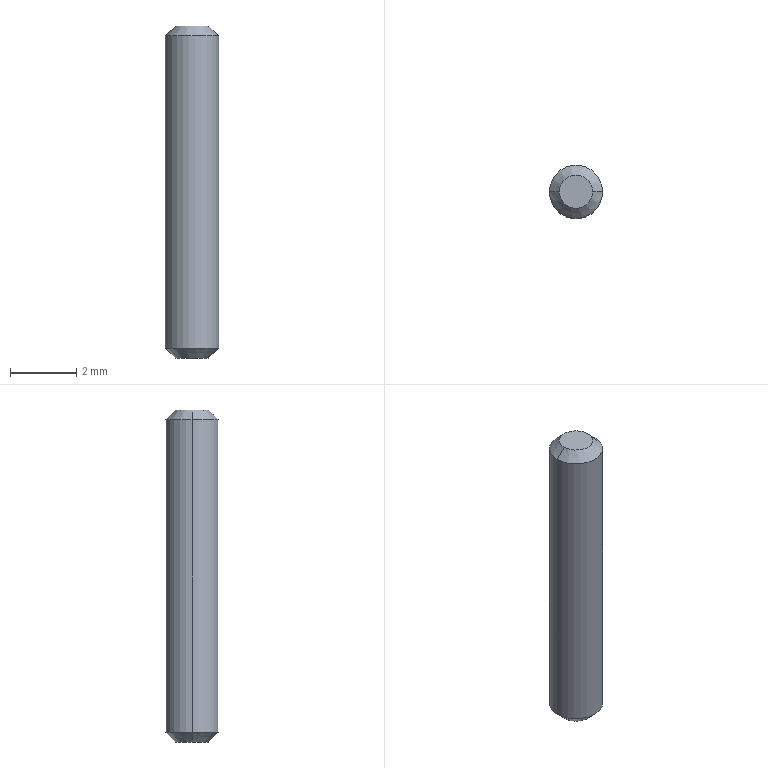Part | STEP file | 1 solid | 8 faces | box 1.6 x 1.6 x 10 mm | volume 19.71 mm3 | cone 4 | cylinder 2 | plane 2 | commonest cylinder face diameters 1.6 x2
STEP:
#1=CARTESIAN_POINT('',(-0.8,0.,9.7));
#2=VERTEX_POINT('',#1);
#3=CARTESIAN_POINT('',(0.8,0.,9.7));
#4=VERTEX_POINT('',#3);
#5=CARTESIAN_POINT('',(0.,0.,9.7));
#6=DIRECTION('',(0.,0.,-1.));
#7=DIRECTION('',(-1.,0.,0.));
#8=AXIS2_PLACEMENT_3D('',#5,#6,#7);
#9=CIRCLE('',#8,0.8);
#10=EDGE_CURVE('',#2,#4,#9,.T.);
#11=ORIENTED_EDGE('',*,*,#10,.T.);
#12=CARTESIAN_POINT('',(0.8,0.,0.3));
#13=VERTEX_POINT('',#12);
#14=CARTESIAN_POINT('',(0.8,0.,10.));
#15=DIRECTION('',(0.,0.,-1.));
#16=VECTOR('',#15,1000.);
#17=LINE('',#14,#16);
#18=EDGE_CURVE('',#4,#13,#17,.T.);
#19=ORIENTED_EDGE('',*,*,#18,.T.);
#20=CARTESIAN_POINT('',(-0.8,0.,0.3));
#21=VERTEX_POINT('',#20);
#22=CARTESIAN_POINT('',(0.,0.,0.3));
#23=DIRECTION('',(0.,0.,1.));
#24=DIRECTION('',(-1.,0.,0.));
#25=AXIS2_PLACEMENT_3D('',#22,#23,#24);
#26=CIRCLE('',#25,0.8);
#27=EDGE_CURVE('',#13,#21,#26,.T.);
#28=ORIENTED_EDGE('',*,*,#27,.T.);
#29=CARTESIAN_POINT('',(-0.8,0.,10.));
#30=DIRECTION('',(0.,0.,-1.));
#31=VECTOR('',#30,1000.);
#32=LINE('',#29,#31);
#33=EDGE_CURVE('',#2,#21,#32,.T.);
#34=ORIENTED_EDGE('',*,*,#33,.F.);
#35=EDGE_LOOP('',(#11,#19,#28,#34));
#36=FACE_OUTER_BOUND('',#35,.T.);
#37=CARTESIAN_POINT('',(0.,0.,10.));
#38=DIRECTION('',(0.,0.,-1.));
#39=DIRECTION('',(-1.,0.,0.));
#40=AXIS2_PLACEMENT_3D('',#37,#38,#39);
#41=CYLINDRICAL_SURFACE('',#40,0.8);
#42=ADVANCED_FACE('',(#36),#41,.T.);
#43=CARTESIAN_POINT('',(0.5,0.,0.));
#44=VERTEX_POINT('',#43);
#45=CARTESIAN_POINT('',(-0.5,0.,0.));
#46=VERTEX_POINT('',#45);
#47=CARTESIAN_POINT('',(0.,0.,0.));
#48=DIRECTION('',(0.,0.,1.));
#49=DIRECTION('',(1.,0.,0.));
#50=AXIS2_PLACEMENT_3D('',#47,#48,#49);
#51=CIRCLE('',#50,0.5);
#52=EDGE_CURVE('',#44,#46,#51,.T.);
#53=ORIENTED_EDGE('',*,*,#52,.T.);
#54=CARTESIAN_POINT('',(-0.8,0.,0.3));
#55=DIRECTION('',(-0.7071,0.,0.7071));
#56=VECTOR('',#55,1000.);
#57=LINE('',#54,#56);
#58=EDGE_CURVE('',#46,#21,#57,.T.);
#59=ORIENTED_EDGE('',*,*,#58,.T.);
#60=ORIENTED_EDGE('',*,*,#27,.F.);
#61=CARTESIAN_POINT('',(0.8,0.,0.3));
#62=DIRECTION('',(0.7071,0.,0.7071));
#63=VECTOR('',#62,1000.);
#64=LINE('',#61,#63);
#65=EDGE_CURVE('',#44,#13,#64,.T.);
#66=ORIENTED_EDGE('',*,*,#65,.F.);
#67=EDGE_LOOP('',(#53,#59,#60,#66));
#68=FACE_OUTER_BOUND('',#67,.T.);
#69=CARTESIAN_POINT('',(0.,0.,0.3));
#70=DIRECTION('',(0.,0.,1.));
#71=DIRECTION('',(1.,0.,0.));
#72=AXIS2_PLACEMENT_3D('',#69,#70,#71);
#73=CONICAL_SURFACE('',#72,0.8,0.7854);
#74=ADVANCED_FACE('',(#68),#73,.T.);
#75=CARTESIAN_POINT('',(-0.5,0.,10.));
#76=VERTEX_POINT('',#75);
#77=CARTESIAN_POINT('',(0.5,0.,10.));
#78=VERTEX_POINT('',#77);
#79=CARTESIAN_POINT('',(0.,0.,10.));
#80=DIRECTION('',(0.,0.,-1.));
#81=DIRECTION('',(-1.,0.,0.));
#82=AXIS2_PLACEMENT_3D('',#79,#80,#81);
#83=CIRCLE('',#82,0.5);
#84=EDGE_CURVE('',#76,#78,#83,.T.);
#85=ORIENTED_EDGE('',*,*,#84,.T.);
#86=CARTESIAN_POINT('',(0.8,0.,9.7));
#87=DIRECTION('',(0.7071,0.,-0.7071));
#88=VECTOR('',#87,1000.);
#89=LINE('',#86,#88);
#90=EDGE_CURVE('',#78,#4,#89,.T.);
#91=ORIENTED_EDGE('',*,*,#90,.T.);
#92=ORIENTED_EDGE('',*,*,#10,.F.);
#93=CARTESIAN_POINT('',(-0.8,0.,9.7));
#94=DIRECTION('',(-0.7071,0.,-0.7071));
#95=VECTOR('',#94,1000.);
#96=LINE('',#93,#95);
#97=EDGE_CURVE('',#76,#2,#96,.T.);
#98=ORIENTED_EDGE('',*,*,#97,.F.);
#99=EDGE_LOOP('',(#85,#91,#92,#98));
#100=FACE_OUTER_BOUND('',#99,.T.);
#101=CARTESIAN_POINT('',(0.,0.,9.7));
#102=DIRECTION('',(0.,0.,-1.));
#103=DIRECTION('',(-1.,0.,0.));
#104=AXIS2_PLACEMENT_3D('',#101,#102,#103);
#105=CONICAL_SURFACE('',#104,0.8,0.7854);
#106=ADVANCED_FACE('',(#100),#105,.T.);
#107=ORIENTED_EDGE('',*,*,#18,.F.);
#108=CARTESIAN_POINT('',(0.,0.,9.7));
#109=DIRECTION('',(0.,0.,-1.));
#110=DIRECTION('',(-1.,0.,0.));
#111=AXIS2_PLACEMENT_3D('',#108,#109,#110);
#112=CIRCLE('',#111,0.8);
#113=EDGE_CURVE('',#4,#2,#112,.T.);
#114=ORIENTED_EDGE('',*,*,#113,.T.);
#115=ORIENTED_EDGE('',*,*,#33,.T.);
#116=CARTESIAN_POINT('',(0.,0.,0.3));
#117=DIRECTION('',(0.,0.,1.));
#118=DIRECTION('',(-1.,0.,0.));
#119=AXIS2_PLACEMENT_3D('',#116,#117,#118);
#120=CIRCLE('',#119,0.8);
#121=EDGE_CURVE('',#21,#13,#120,.T.);
#122=ORIENTED_EDGE('',*,*,#121,.T.);
#123=EDGE_LOOP('',(#107,#114,#115,#122));
#124=FACE_OUTER_BOUND('',#123,.T.);
#125=CARTESIAN_POINT('',(0.,0.,10.));
#126=DIRECTION('',(0.,0.,-1.));
#127=DIRECTION('',(-1.,0.,0.));
#128=AXIS2_PLACEMENT_3D('',#125,#126,#127);
#129=CYLINDRICAL_SURFACE('',#128,0.8);
#130=ADVANCED_FACE('',(#124),#129,.T.);
#131=ORIENTED_EDGE('',*,*,#58,.F.);
#132=CARTESIAN_POINT('',(0.,0.,0.));
#133=DIRECTION('',(0.,0.,1.));
#134=DIRECTION('',(1.,0.,0.));
#135=AXIS2_PLACEMENT_3D('',#132,#133,#134);
#136=CIRCLE('',#135,0.5);
#137=EDGE_CURVE('',#46,#44,#136,.T.);
#138=ORIENTED_EDGE('',*,*,#137,.T.);
#139=ORIENTED_EDGE('',*,*,#65,.T.);
#140=ORIENTED_EDGE('',*,*,#121,.F.);
#141=EDGE_LOOP('',(#131,#138,#139,#140));
#142=FACE_OUTER_BOUND('',#141,.T.);
#143=CARTESIAN_POINT('',(0.,0.,0.3));
#144=DIRECTION('',(0.,0.,1.));
#145=DIRECTION('',(1.,0.,0.));
#146=AXIS2_PLACEMENT_3D('',#143,#144,#145);
#147=CONICAL_SURFACE('',#146,0.8,0.7854);
#148=ADVANCED_FACE('',(#142),#147,.T.);
#149=ORIENTED_EDGE('',*,*,#90,.F.);
#150=CARTESIAN_POINT('',(0.,0.,10.));
#151=DIRECTION('',(0.,0.,-1.));
#152=DIRECTION('',(-1.,0.,0.));
#153=AXIS2_PLACEMENT_3D('',#150,#151,#152);
#154=CIRCLE('',#153,0.5);
#155=EDGE_CURVE('',#78,#76,#154,.T.);
#156=ORIENTED_EDGE('',*,*,#155,.T.);
#157=ORIENTED_EDGE('',*,*,#97,.T.);
#158=ORIENTED_EDGE('',*,*,#113,.F.);
#159=EDGE_LOOP('',(#149,#156,#157,#158));
#160=FACE_OUTER_BOUND('',#159,.T.);
#161=CARTESIAN_POINT('',(0.,0.,9.7));
#162=DIRECTION('',(0.,0.,-1.));
#163=DIRECTION('',(-1.,0.,0.));
#164=AXIS2_PLACEMENT_3D('',#161,#162,#163);
#165=CONICAL_SURFACE('',#164,0.8,0.7854);
#166=ADVANCED_FACE('',(#160),#165,.T.);
#167=ORIENTED_EDGE('',*,*,#52,.F.);
#168=ORIENTED_EDGE('',*,*,#137,.F.);
#169=EDGE_LOOP('',(#167,#168));
#170=FACE_OUTER_BOUND('',#169,.T.);
#171=CARTESIAN_POINT('',(0.,0.,0.));
#172=DIRECTION('',(0.,0.,1.));
#173=DIRECTION('',(1.,0.,0.));
#174=AXIS2_PLACEMENT_3D('',#171,#172,#173);
#175=PLANE('',#174);
#176=ADVANCED_FACE('',(#170),#175,.F.);
#177=ORIENTED_EDGE('',*,*,#84,.F.);
#178=ORIENTED_EDGE('',*,*,#155,.F.);
#179=EDGE_LOOP('',(#177,#178));
#180=FACE_OUTER_BOUND('',#179,.T.);
#181=CARTESIAN_POINT('',(0.,0.,10.));
#182=DIRECTION('',(0.,0.,1.));
#183=DIRECTION('',(1.,0.,0.));
#184=AXIS2_PLACEMENT_3D('',#181,#182,#183);
#185=PLANE('',#184);
#186=ADVANCED_FACE('',(#180),#185,.T.);
#187=CLOSED_SHELL('',(#42,#74,#106,#130,#148,#166,#176,#186));
#188=MANIFOLD_SOLID_BREP('',#187);
#189=CARTESIAN_POINT('',(0.,0.,0.));
#190=DIRECTION('',(0.,0.,1.));
#191=DIRECTION('',(1.,0.,0.));
#192=AXIS2_PLACEMENT_3D('',#189,#190,#191);
#193=(LENGTH_UNIT()NAMED_UNIT(*)SI_UNIT(.MILLI.,.METRE.));
#194=UNCERTAINTY_MEASURE_WITH_UNIT(LENGTH_MEASURE(0.00001),#193,'','');
#195=(NAMED_UNIT(*)PLANE_ANGLE_UNIT()SI_UNIT($,.RADIAN.));
#196=(NAMED_UNIT(*)SI_UNIT($,.STERADIAN.)SOLID_ANGLE_UNIT());
#197=(GEOMETRIC_REPRESENTATION_CONTEXT(3)GLOBAL_UNCERTAINTY_ASSIGNED_CONTEXT((#194))GLOBAL_UNIT_ASSIGNED_CONTEXT((#193,#195,#196))REPRESENTATION_CONTEXT('',''));
#198=ADVANCED_BREP_SHAPE_REPRESENTATION('',(#188,#192),#197);